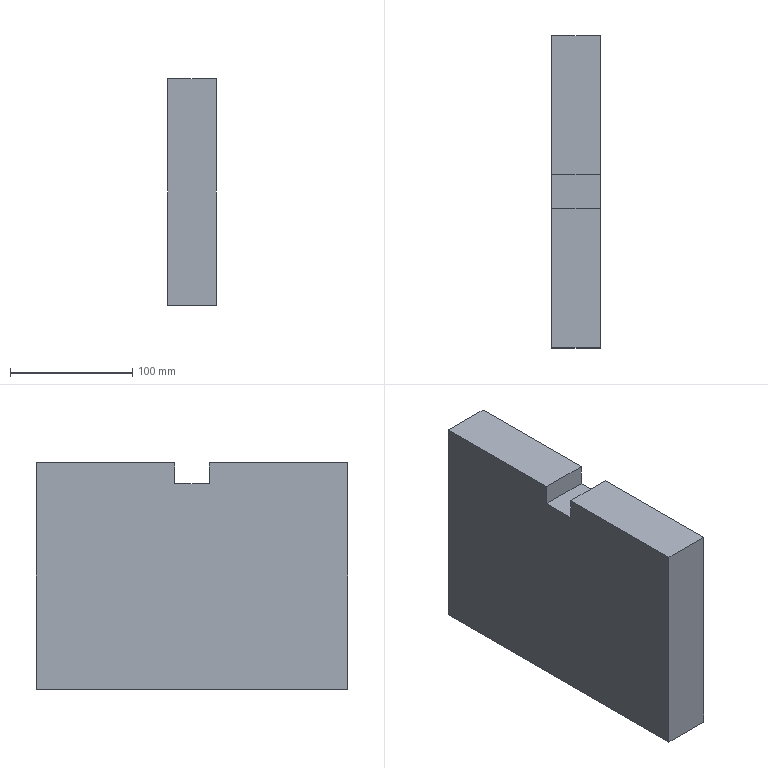Part | STEP file | 1 solid | 14 faces | box 40 x 255 x 185 mm | volume 1855337 mm3 | plane 10 | cylinder 2 | cone 2 | commonest cylinder face diameters 14 x2
STEP:
#1=CARTESIAN_POINT('',(170.,-14.,-124.));
#2=VERTEX_POINT('',#1);
#3=CARTESIAN_POINT('',(170.,-14.,-107.));
#4=VERTEX_POINT('',#3);
#5=CARTESIAN_POINT('',(170.,-14.,-122.));
#6=DIRECTION('',(0.,0.,1.));
#7=VECTOR('',#6,1.);
#8=LINE('',#5,#7);
#9=EDGE_CURVE('',#2,#4,#8,.T.);
#10=ORIENTED_EDGE('',*,*,#9,.F.);
#11=CARTESIAN_POINT('',(170.,14.,-124.));
#12=VERTEX_POINT('',#11);
#13=CARTESIAN_POINT('',(170.,-1.,-124.));
#14=DIRECTION('',(0.,-1.,0.));
#15=VECTOR('',#14,1.);
#16=LINE('',#13,#15);
#17=EDGE_CURVE('',#12,#2,#16,.T.);
#18=ORIENTED_EDGE('',*,*,#17,.F.);
#19=CARTESIAN_POINT('',(170.,14.,-107.));
#20=VERTEX_POINT('',#19);
#21=CARTESIAN_POINT('',(170.,14.,-107.));
#22=DIRECTION('',(0.,0.,1.));
#23=VECTOR('',#22,1.);
#24=LINE('',#21,#23);
#25=EDGE_CURVE('',#12,#20,#24,.T.);
#26=ORIENTED_EDGE('',*,*,#25,.T.);
#27=CARTESIAN_POINT('',(170.,127.5,-107.));
#28=VERTEX_POINT('',#27);
#29=CARTESIAN_POINT('',(170.,-1.,-107.));
#30=DIRECTION('',(0.,-1.,0.));
#31=VECTOR('',#30,1.);
#32=LINE('',#29,#31);
#33=EDGE_CURVE('',#28,#20,#32,.T.);
#34=ORIENTED_EDGE('',*,*,#33,.F.);
#35=CARTESIAN_POINT('',(170.,127.5,-292.));
#36=VERTEX_POINT('',#35);
#37=CARTESIAN_POINT('',(170.,127.5,-107.));
#38=DIRECTION('',(0.,0.,1.));
#39=VECTOR('',#38,1.);
#40=LINE('',#37,#39);
#41=EDGE_CURVE('',#36,#28,#40,.T.);
#42=ORIENTED_EDGE('',*,*,#41,.F.);
#43=CARTESIAN_POINT('',(170.,-127.5,-292.));
#44=VERTEX_POINT('',#43);
#45=CARTESIAN_POINT('',(170.,-1.,-292.));
#46=DIRECTION('',(0.,-1.,0.));
#47=VECTOR('',#46,1.);
#48=LINE('',#45,#47);
#49=EDGE_CURVE('',#36,#44,#48,.T.);
#50=ORIENTED_EDGE('',*,*,#49,.T.);
#51=CARTESIAN_POINT('',(170.,-127.5,-107.));
#52=VERTEX_POINT('',#51);
#53=CARTESIAN_POINT('',(170.,-127.5,-107.));
#54=DIRECTION('',(0.,0.,1.));
#55=VECTOR('',#54,1.);
#56=LINE('',#53,#55);
#57=EDGE_CURVE('',#44,#52,#56,.T.);
#58=ORIENTED_EDGE('',*,*,#57,.T.);
#59=CARTESIAN_POINT('',(170.,-1.,-107.));
#60=DIRECTION('',(0.,-1.,0.));
#61=VECTOR('',#60,1.);
#62=LINE('',#59,#61);
#63=EDGE_CURVE('',#4,#52,#62,.T.);
#64=ORIENTED_EDGE('',*,*,#63,.F.);
#65=EDGE_LOOP('',(#10,#18,#26,#34,#42,#50,#58,#64));
#66=FACE_OUTER_BOUND('',#65,.T.);
#67=CARTESIAN_POINT('',(170.,-1.,-107.));
#68=DIRECTION('',(-1.,0.,0.));
#69=DIRECTION('',(0.,-1.,0.));
#70=AXIS2_PLACEMENT_3D('',#67,#68,#69);
#71=PLANE('',#70);
#72=ADVANCED_FACE('',(#66),#71,.T.);
#73=CARTESIAN_POINT('',(210.,14.,-124.));
#74=VERTEX_POINT('',#73);
#75=CARTESIAN_POINT('',(210.,14.,-107.));
#76=VERTEX_POINT('',#75);
#77=CARTESIAN_POINT('',(210.,14.,-122.));
#78=DIRECTION('',(0.,0.,1.));
#79=VECTOR('',#78,1.);
#80=LINE('',#77,#79);
#81=EDGE_CURVE('',#74,#76,#80,.T.);
#82=ORIENTED_EDGE('',*,*,#81,.F.);
#83=CARTESIAN_POINT('',(210.,-14.,-124.));
#84=VERTEX_POINT('',#83);
#85=CARTESIAN_POINT('',(210.,-1.,-124.));
#86=DIRECTION('',(0.,1.,0.));
#87=VECTOR('',#86,1.);
#88=LINE('',#85,#87);
#89=EDGE_CURVE('',#84,#74,#88,.T.);
#90=ORIENTED_EDGE('',*,*,#89,.F.);
#91=CARTESIAN_POINT('',(210.,-14.,-107.));
#92=VERTEX_POINT('',#91);
#93=CARTESIAN_POINT('',(210.,-14.,-107.));
#94=DIRECTION('',(0.,0.,1.));
#95=VECTOR('',#94,1.);
#96=LINE('',#93,#95);
#97=EDGE_CURVE('',#84,#92,#96,.T.);
#98=ORIENTED_EDGE('',*,*,#97,.T.);
#99=CARTESIAN_POINT('',(210.,-127.5,-107.));
#100=VERTEX_POINT('',#99);
#101=CARTESIAN_POINT('',(210.,-1.,-107.));
#102=DIRECTION('',(0.,1.,0.));
#103=VECTOR('',#102,1.);
#104=LINE('',#101,#103);
#105=EDGE_CURVE('',#100,#92,#104,.T.);
#106=ORIENTED_EDGE('',*,*,#105,.F.);
#107=CARTESIAN_POINT('',(210.,-127.5,-292.));
#108=VERTEX_POINT('',#107);
#109=CARTESIAN_POINT('',(210.,-127.5,-107.));
#110=DIRECTION('',(0.,0.,1.));
#111=VECTOR('',#110,1.);
#112=LINE('',#109,#111);
#113=EDGE_CURVE('',#108,#100,#112,.T.);
#114=ORIENTED_EDGE('',*,*,#113,.F.);
#115=CARTESIAN_POINT('',(210.,127.5,-292.));
#116=VERTEX_POINT('',#115);
#117=CARTESIAN_POINT('',(210.,-1.,-292.));
#118=DIRECTION('',(0.,1.,0.));
#119=VECTOR('',#118,1.);
#120=LINE('',#117,#119);
#121=EDGE_CURVE('',#108,#116,#120,.T.);
#122=ORIENTED_EDGE('',*,*,#121,.T.);
#123=CARTESIAN_POINT('',(210.,127.5,-107.));
#124=VERTEX_POINT('',#123);
#125=CARTESIAN_POINT('',(210.,127.5,-107.));
#126=DIRECTION('',(0.,0.,1.));
#127=VECTOR('',#126,1.);
#128=LINE('',#125,#127);
#129=EDGE_CURVE('',#116,#124,#128,.T.);
#130=ORIENTED_EDGE('',*,*,#129,.T.);
#131=CARTESIAN_POINT('',(210.,-1.,-107.));
#132=DIRECTION('',(0.,1.,0.));
#133=VECTOR('',#132,1.);
#134=LINE('',#131,#133);
#135=EDGE_CURVE('',#76,#124,#134,.T.);
#136=ORIENTED_EDGE('',*,*,#135,.F.);
#137=EDGE_LOOP('',(#82,#90,#98,#106,#114,#122,#130,#136));
#138=FACE_OUTER_BOUND('',#137,.T.);
#139=CARTESIAN_POINT('',(210.,-1.,-107.));
#140=DIRECTION('',(1.,0.,0.));
#141=DIRECTION('',(0.,1.,0.));
#142=AXIS2_PLACEMENT_3D('',#139,#140,#141);
#143=PLANE('',#142);
#144=ADVANCED_FACE('',(#138),#143,.T.);
#145=CARTESIAN_POINT('',(628.5,-14.,-107.));
#146=DIRECTION('',(1.,0.,0.));
#147=VECTOR('',#146,1.);
#148=LINE('',#145,#147);
#149=EDGE_CURVE('',#4,#92,#148,.T.);
#150=ORIENTED_EDGE('',*,*,#149,.F.);
#151=ORIENTED_EDGE('',*,*,#63,.T.);
#152=CARTESIAN_POINT('',(628.5,-127.5,-107.));
#153=DIRECTION('',(1.,0.,0.));
#154=VECTOR('',#153,1.);
#155=LINE('',#152,#154);
#156=EDGE_CURVE('',#52,#100,#155,.T.);
#157=ORIENTED_EDGE('',*,*,#156,.T.);
#158=ORIENTED_EDGE('',*,*,#105,.T.);
#159=EDGE_LOOP('',(#150,#151,#157,#158));
#160=FACE_OUTER_BOUND('',#159,.T.);
#161=CARTESIAN_POINT('',(628.5,-1.,-107.));
#162=DIRECTION('',(0.,0.,1.));
#163=DIRECTION('',(1.,0.,0.));
#164=AXIS2_PLACEMENT_3D('',#161,#162,#163);
#165=PLANE('',#164);
#166=ADVANCED_FACE('',(#160),#165,.T.);
#167=ORIENTED_EDGE('',*,*,#41,.T.);
#168=CARTESIAN_POINT('',(628.5,127.5,-107.));
#169=DIRECTION('',(-1.,0.,0.));
#170=VECTOR('',#169,1.);
#171=LINE('',#168,#170);
#172=EDGE_CURVE('',#124,#28,#171,.T.);
#173=ORIENTED_EDGE('',*,*,#172,.F.);
#174=ORIENTED_EDGE('',*,*,#129,.F.);
#175=CARTESIAN_POINT('',(628.5,127.5,-292.));
#176=DIRECTION('',(-1.,0.,0.));
#177=VECTOR('',#176,1.);
#178=LINE('',#175,#177);
#179=EDGE_CURVE('',#116,#36,#178,.T.);
#180=ORIENTED_EDGE('',*,*,#179,.T.);
#181=EDGE_LOOP('',(#167,#173,#174,#180));
#182=FACE_OUTER_BOUND('',#181,.T.);
#183=CARTESIAN_POINT('',(628.5,127.5,-107.));
#184=DIRECTION('',(0.,1.,0.));
#185=DIRECTION('',(-1.,0.,0.));
#186=AXIS2_PLACEMENT_3D('',#183,#184,#185);
#187=PLANE('',#186);
#188=ADVANCED_FACE('',(#182),#187,.T.);
#189=CARTESIAN_POINT('',(628.5,-127.5,-292.));
#190=DIRECTION('',(1.,0.,0.));
#191=VECTOR('',#190,1.);
#192=LINE('',#189,#191);
#193=EDGE_CURVE('',#44,#108,#192,.T.);
#194=ORIENTED_EDGE('',*,*,#193,.T.);
#195=ORIENTED_EDGE('',*,*,#113,.T.);
#196=ORIENTED_EDGE('',*,*,#156,.F.);
#197=ORIENTED_EDGE('',*,*,#57,.F.);
#198=EDGE_LOOP('',(#194,#195,#196,#197));
#199=FACE_OUTER_BOUND('',#198,.T.);
#200=CARTESIAN_POINT('',(628.5,-127.5,-107.));
#201=DIRECTION('',(0.,-1.,0.));
#202=DIRECTION('',(1.,0.,0.));
#203=AXIS2_PLACEMENT_3D('',#200,#201,#202);
#204=PLANE('',#203);
#205=ADVANCED_FACE('',(#199),#204,.T.);
#206=CARTESIAN_POINT('',(628.5,14.,-107.));
#207=DIRECTION('',(-1.,0.,0.));
#208=VECTOR('',#207,1.);
#209=LINE('',#206,#208);
#210=EDGE_CURVE('',#76,#20,#209,.T.);
#211=ORIENTED_EDGE('',*,*,#210,.F.);
#212=ORIENTED_EDGE('',*,*,#135,.T.);
#213=ORIENTED_EDGE('',*,*,#172,.T.);
#214=ORIENTED_EDGE('',*,*,#33,.T.);
#215=EDGE_LOOP('',(#211,#212,#213,#214));
#216=FACE_OUTER_BOUND('',#215,.T.);
#217=CARTESIAN_POINT('',(628.5,-1.,-107.));
#218=DIRECTION('',(0.,0.,1.));
#219=DIRECTION('',(1.,0.,0.));
#220=AXIS2_PLACEMENT_3D('',#217,#218,#219);
#221=PLANE('',#220);
#222=ADVANCED_FACE('',(#216),#221,.T.);
#223=ORIENTED_EDGE('',*,*,#121,.F.);
#224=ORIENTED_EDGE('',*,*,#193,.F.);
#225=ORIENTED_EDGE('',*,*,#49,.F.);
#226=ORIENTED_EDGE('',*,*,#179,.F.);
#227=EDGE_LOOP('',(#223,#224,#225,#226));
#228=FACE_BOUND('',#227,.T.);
#229=CARTESIAN_POINT('',(197.,102.5,-292.));
#230=VERTEX_POINT('',#229);
#231=CARTESIAN_POINT('',(190.,102.5,-292.));
#232=DIRECTION('',(0.,0.,1.));
#233=DIRECTION('',(1.,0.,0.));
#234=AXIS2_PLACEMENT_3D('',#231,#232,#233);
#235=CIRCLE('',#234,7.);
#236=EDGE_CURVE('',#230,#230,#235,.T.);
#237=ORIENTED_EDGE('',*,*,#236,.T.);
#238=EDGE_LOOP('',(#237));
#239=FACE_BOUND('',#238,.T.);
#240=CARTESIAN_POINT('',(197.,-102.5,-292.));
#241=VERTEX_POINT('',#240);
#242=CARTESIAN_POINT('',(190.,-102.5,-292.));
#243=DIRECTION('',(0.,0.,-1.));
#244=DIRECTION('',(1.,0.,0.));
#245=AXIS2_PLACEMENT_3D('',#242,#243,#244);
#246=CIRCLE('',#245,7.);
#247=EDGE_CURVE('',#241,#241,#246,.T.);
#248=ORIENTED_EDGE('',*,*,#247,.F.);
#249=EDGE_LOOP('',(#248));
#250=FACE_BOUND('',#249,.T.);
#251=CARTESIAN_POINT('',(618.5,-1.,-292.));
#252=DIRECTION('',(0.,0.,-1.));
#253=DIRECTION('',(1.,0.,0.));
#254=AXIS2_PLACEMENT_3D('',#251,#252,#253);
#255=PLANE('',#254);
#256=ADVANCED_FACE('',(#228,#239,#250),#255,.T.);
#257=ORIENTED_EDGE('',*,*,#149,.T.);
#258=ORIENTED_EDGE('',*,*,#97,.F.);
#259=CARTESIAN_POINT('',(190.919,-14.,-124.));
#260=DIRECTION('',(-1.,0.,0.));
#261=VECTOR('',#260,1.);
#262=LINE('',#259,#261);
#263=EDGE_CURVE('',#84,#2,#262,.T.);
#264=ORIENTED_EDGE('',*,*,#263,.T.);
#265=ORIENTED_EDGE('',*,*,#9,.T.);
#266=EDGE_LOOP('',(#257,#258,#264,#265));
#267=FACE_OUTER_BOUND('',#266,.T.);
#268=CARTESIAN_POINT('',(190.919,-14.,-122.));
#269=DIRECTION('',(0.,-1.,0.));
#270=DIRECTION('',(0.,0.,-1.));
#271=AXIS2_PLACEMENT_3D('',#268,#269,#270);
#272=PLANE('',#271);
#273=ADVANCED_FACE('',(#267),#272,.F.);
#274=ORIENTED_EDGE('',*,*,#210,.T.);
#275=ORIENTED_EDGE('',*,*,#25,.F.);
#276=CARTESIAN_POINT('',(190.919,14.,-124.));
#277=DIRECTION('',(1.,0.,0.));
#278=VECTOR('',#277,1.);
#279=LINE('',#276,#278);
#280=EDGE_CURVE('',#12,#74,#279,.T.);
#281=ORIENTED_EDGE('',*,*,#280,.T.);
#282=ORIENTED_EDGE('',*,*,#81,.T.);
#283=EDGE_LOOP('',(#274,#275,#281,#282));
#284=FACE_OUTER_BOUND('',#283,.T.);
#285=CARTESIAN_POINT('',(190.919,14.,-122.));
#286=DIRECTION('',(0.,1.,0.));
#287=DIRECTION('',(0.,0.,1.));
#288=AXIS2_PLACEMENT_3D('',#285,#286,#287);
#289=PLANE('',#288);
#290=ADVANCED_FACE('',(#284),#289,.F.);
#291=ORIENTED_EDGE('',*,*,#89,.T.);
#292=ORIENTED_EDGE('',*,*,#280,.F.);
#293=ORIENTED_EDGE('',*,*,#17,.T.);
#294=ORIENTED_EDGE('',*,*,#263,.F.);
#295=EDGE_LOOP('',(#291,#292,#293,#294));
#296=FACE_OUTER_BOUND('',#295,.T.);
#297=CARTESIAN_POINT('',(190.919,0.,-124.));
#298=DIRECTION('',(0.,0.,-1.));
#299=DIRECTION('',(-1.,0.,0.));
#300=AXIS2_PLACEMENT_3D('',#297,#298,#299);
#301=PLANE('',#300);
#302=ADVANCED_FACE('',(#296),#301,.F.);
#303=CARTESIAN_POINT('',(183.,102.5,-252.));
#304=VERTEX_POINT('',#303);
#305=CARTESIAN_POINT('',(190.,102.5,-252.));
#306=DIRECTION('',(0.,0.,-1.));
#307=DIRECTION('',(-1.,0.,0.));
#308=AXIS2_PLACEMENT_3D('',#305,#306,#307);
#309=CIRCLE('',#308,7.);
#310=EDGE_CURVE('',#304,#304,#309,.T.);
#311=ORIENTED_EDGE('',*,*,#310,.F.);
#312=EDGE_LOOP('',(#311));
#313=FACE_BOUND('',#312,.T.);
#314=ORIENTED_EDGE('',*,*,#236,.F.);
#315=EDGE_LOOP('',(#314));
#316=FACE_BOUND('',#315,.T.);
#317=CARTESIAN_POINT('',(190.,102.5,-292.));
#318=DIRECTION('',(0.,0.,1.));
#319=DIRECTION('',(-1.,0.,0.));
#320=AXIS2_PLACEMENT_3D('',#317,#318,#319);
#321=CYLINDRICAL_SURFACE('',#320,7.);
#322=ADVANCED_FACE('',(#313,#316),#321,.F.);
#323=ORIENTED_EDGE('',*,*,#310,.T.);
#324=EDGE_LOOP('',(#323));
#325=FACE_BOUND('',#324,.T.);
#326=CARTESIAN_POINT('',(190.,102.5,-249.));
#327=VERTEX_POINT('',#326);
#328=VERTEX_LOOP('',#327);
#329=FACE_BOUND('',#328,.T.);
#330=CARTESIAN_POINT('',(190.,102.5,-249.));
#331=DIRECTION('',(0.,0.,-1.));
#332=DIRECTION('',(-1.,0.,0.));
#333=AXIS2_PLACEMENT_3D('',#330,#331,#332);
#334=CONICAL_SURFACE('',#333,0.,66.801);
#335=ADVANCED_FACE('',(#325,#329),#334,.F.);
#336=CARTESIAN_POINT('',(183.,-102.5,-252.));
#337=VERTEX_POINT('',#336);
#338=CARTESIAN_POINT('',(190.,-102.5,-252.));
#339=DIRECTION('',(0.,0.,1.));
#340=DIRECTION('',(-1.,0.,0.));
#341=AXIS2_PLACEMENT_3D('',#338,#339,#340);
#342=CIRCLE('',#341,7.);
#343=EDGE_CURVE('',#337,#337,#342,.T.);
#344=ORIENTED_EDGE('',*,*,#343,.T.);
#345=EDGE_LOOP('',(#344));
#346=FACE_BOUND('',#345,.T.);
#347=ORIENTED_EDGE('',*,*,#247,.T.);
#348=EDGE_LOOP('',(#347));
#349=FACE_BOUND('',#348,.T.);
#350=CARTESIAN_POINT('',(190.,-102.5,-292.));
#351=DIRECTION('',(0.,0.,1.));
#352=DIRECTION('',(-1.,0.,0.));
#353=AXIS2_PLACEMENT_3D('',#350,#351,#352);
#354=CYLINDRICAL_SURFACE('',#353,7.);
#355=ADVANCED_FACE('',(#346,#349),#354,.F.);
#356=ORIENTED_EDGE('',*,*,#343,.F.);
#357=EDGE_LOOP('',(#356));
#358=FACE_BOUND('',#357,.T.);
#359=CARTESIAN_POINT('',(190.,-102.5,-249.));
#360=VERTEX_POINT('',#359);
#361=VERTEX_LOOP('',#360);
#362=FACE_BOUND('',#361,.T.);
#363=CARTESIAN_POINT('',(190.,-102.5,-249.));
#364=DIRECTION('',(0.,0.,-1.));
#365=DIRECTION('',(-1.,0.,0.));
#366=AXIS2_PLACEMENT_3D('',#363,#364,#365);
#367=CONICAL_SURFACE('',#366,0.,66.801);
#368=ADVANCED_FACE('',(#358,#362),#367,.F.);
#369=CLOSED_SHELL('',(#72,#144,#166,#188,#205,#222,#256,#273,#290,#302,#322,#335,#355,#368));
#370=MANIFOLD_SOLID_BREP('',#369);
#371=(LENGTH_UNIT()NAMED_UNIT(*)SI_UNIT(.MILLI.,.METRE.));
#372=UNCERTAINTY_MEASURE_WITH_UNIT(LENGTH_MEASURE(0.00002),#371,'','');
#373=(NAMED_UNIT(*)PLANE_ANGLE_UNIT()SI_UNIT($,.RADIAN.));
#374=PLANE_ANGLE_MEASURE_WITH_UNIT(PLANE_ANGLE_MEASURE(0.01745),#373);
#375=DIMENSIONAL_EXPONENTS(0.,0.,0.,0.,0.,0.,0.);
#376=(CONVERSION_BASED_UNIT('DEGREE',#374)NAMED_UNIT(#375)PLANE_ANGLE_UNIT());
#377=(NAMED_UNIT(*)SI_UNIT($,.STERADIAN.)SOLID_ANGLE_UNIT());
#378=(GEOMETRIC_REPRESENTATION_CONTEXT(3)GLOBAL_UNCERTAINTY_ASSIGNED_CONTEXT((#372))GLOBAL_UNIT_ASSIGNED_CONTEXT((#371,#376,#377))REPRESENTATION_CONTEXT('',''));
#379=ADVANCED_BREP_SHAPE_REPRESENTATION('',(#370),#378);